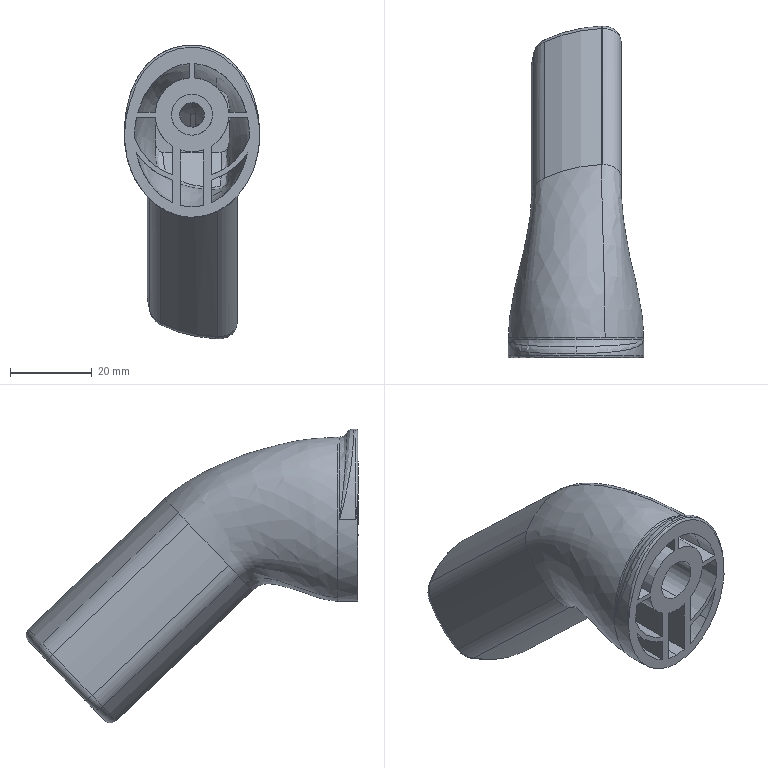Part | SolidWorks | features BaseBody 1 | 1 solid | 161 faces | box 33 x 80.996 x 71.706 mm | volume 27691 mm3 | plane 49 | spline 47 | cylinder 45 | torus 20 | commonest cylinder face diameters 4 x6 18 x6 6 x5 2 x3 9 x3 5.5 x2